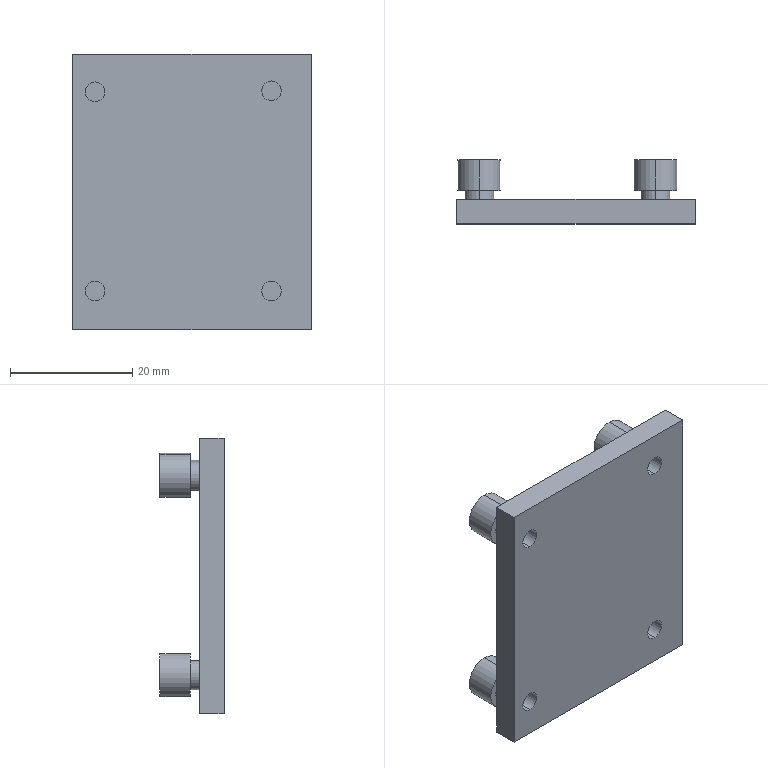Part | SolidWorks | features BaseBody 1 | 1 solid | 70 faces | box 39 x 10.5 x 45 mm | volume 7555 mm3 | plane 46 | cylinder 24 | commonest cylinder face diameters 3.211 x8 4.755 x8 7 x8